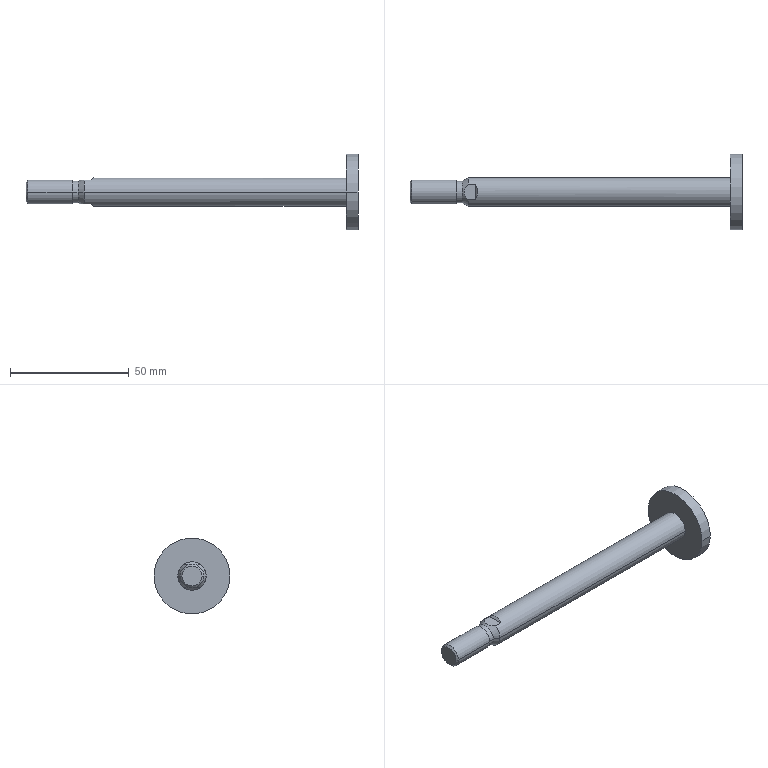Part | SolidWorks | features BaseBody 1 | 1 solid | 20 faces | box 140 x 32 x 32 mm | volume 18387 mm3 | cylinder 8 | plane 8 | cone 4 | commonest cylinder face diameters 9.1 x2 10 x2 12 x2 32 x2
STEP:
#1=CARTESIAN_POINT('',(-40.,4.233,0.));
#2=VERTEX_POINT('',#1);
#3=CARTESIAN_POINT('',(-40.,-4.233,0.));
#4=VERTEX_POINT('',#3);
#5=CARTESIAN_POINT('',(-40.,0.,0.));
#6=DIRECTION('',(1.,0.,0.));
#7=DIRECTION('',(0.,1.,0.));
#8=AXIS2_PLACEMENT_3D('',#5,#6,#7);
#9=CIRCLE('',#8,4.233);
#10=EDGE_CURVE('',#2,#4,#9,.T.);
#11=ORIENTED_EDGE('',*,*,#10,.T.);
#12=CARTESIAN_POINT('',(-39.233,-5.,0.));
#13=VERTEX_POINT('',#12);
#14=CARTESIAN_POINT('',(-40.,-4.233,0.));
#15=DIRECTION('',(0.7071,-0.7071,0.));
#16=VECTOR('',#15,1000.);
#17=LINE('',#14,#16);
#18=EDGE_CURVE('',#4,#13,#17,.T.);
#19=ORIENTED_EDGE('',*,*,#18,.T.);
#20=CARTESIAN_POINT('',(-39.233,5.,0.));
#21=VERTEX_POINT('',#20);
#22=CARTESIAN_POINT('',(-39.233,0.,0.));
#23=DIRECTION('',(1.,0.,0.));
#24=DIRECTION('',(0.,1.,0.));
#25=AXIS2_PLACEMENT_3D('',#22,#23,#24);
#26=CIRCLE('',#25,5.);
#27=EDGE_CURVE('',#21,#13,#26,.T.);
#28=ORIENTED_EDGE('',*,*,#27,.F.);
#29=CARTESIAN_POINT('',(-40.,4.233,0.));
#30=DIRECTION('',(0.7071,0.7071,0.));
#31=VECTOR('',#30,1000.);
#32=LINE('',#29,#31);
#33=EDGE_CURVE('',#2,#21,#32,.T.);
#34=ORIENTED_EDGE('',*,*,#33,.F.);
#35=EDGE_LOOP('',(#11,#19,#28,#34));
#36=FACE_OUTER_BOUND('',#35,.T.);
#37=CARTESIAN_POINT('',(-40.,0.,0.));
#38=DIRECTION('',(1.,0.,0.));
#39=DIRECTION('',(0.,1.,0.));
#40=AXIS2_PLACEMENT_3D('',#37,#38,#39);
#41=CONICAL_SURFACE('',#40,4.233,0.7854);
#42=ADVANCED_FACE('',(#36),#41,.T.);
#43=ORIENTED_EDGE('',*,*,#27,.T.);
#44=CARTESIAN_POINT('',(-20.5,-5.,0.));
#45=VERTEX_POINT('',#44);
#46=CARTESIAN_POINT('',(100.,-5.,0.));
#47=DIRECTION('',(1.,0.,0.));
#48=VECTOR('',#47,1000.);
#49=LINE('',#46,#48);
#50=EDGE_CURVE('',#13,#45,#49,.T.);
#51=ORIENTED_EDGE('',*,*,#50,.T.);
#52=CARTESIAN_POINT('',(-20.5,5.,0.));
#53=VERTEX_POINT('',#52);
#54=CARTESIAN_POINT('',(-20.5,0.,0.));
#55=DIRECTION('',(1.,0.,0.));
#56=DIRECTION('',(0.,1.,0.));
#57=AXIS2_PLACEMENT_3D('',#54,#55,#56);
#58=CIRCLE('',#57,5.);
#59=EDGE_CURVE('',#53,#45,#58,.T.);
#60=ORIENTED_EDGE('',*,*,#59,.F.);
#61=CARTESIAN_POINT('',(100.,5.,0.));
#62=DIRECTION('',(1.,0.,0.));
#63=VECTOR('',#62,1000.);
#64=LINE('',#61,#63);
#65=EDGE_CURVE('',#21,#53,#64,.T.);
#66=ORIENTED_EDGE('',*,*,#65,.F.);
#67=EDGE_LOOP('',(#43,#51,#60,#66));
#68=FACE_OUTER_BOUND('',#67,.T.);
#69=CARTESIAN_POINT('',(100.,0.,0.));
#70=DIRECTION('',(1.,0.,0.));
#71=DIRECTION('',(0.,1.,0.));
#72=AXIS2_PLACEMENT_3D('',#69,#70,#71);
#73=CYLINDRICAL_SURFACE('',#72,5.);
#74=ADVANCED_FACE('',(#68),#73,.T.);
#75=CARTESIAN_POINT('',(95.,16.,0.));
#76=VERTEX_POINT('',#75);
#77=CARTESIAN_POINT('',(95.,-16.,0.));
#78=VERTEX_POINT('',#77);
#79=CARTESIAN_POINT('',(95.,0.,0.));
#80=DIRECTION('',(1.,0.,0.));
#81=DIRECTION('',(0.,1.,0.));
#82=AXIS2_PLACEMENT_3D('',#79,#80,#81);
#83=CIRCLE('',#82,16.);
#84=EDGE_CURVE('',#76,#78,#83,.T.);
#85=ORIENTED_EDGE('',*,*,#84,.T.);
#86=CARTESIAN_POINT('',(100.,-16.,0.));
#87=VERTEX_POINT('',#86);
#88=CARTESIAN_POINT('',(100.,-16.,0.));
#89=DIRECTION('',(1.,0.,0.));
#90=VECTOR('',#89,1000.);
#91=LINE('',#88,#90);
#92=EDGE_CURVE('',#78,#87,#91,.T.);
#93=ORIENTED_EDGE('',*,*,#92,.T.);
#94=CARTESIAN_POINT('',(100.,16.,0.));
#95=VERTEX_POINT('',#94);
#96=CARTESIAN_POINT('',(100.,0.,0.));
#97=DIRECTION('',(1.,0.,0.));
#98=DIRECTION('',(0.,1.,0.));
#99=AXIS2_PLACEMENT_3D('',#96,#97,#98);
#100=CIRCLE('',#99,16.);
#101=EDGE_CURVE('',#95,#87,#100,.T.);
#102=ORIENTED_EDGE('',*,*,#101,.F.);
#103=CARTESIAN_POINT('',(100.,16.,0.));
#104=DIRECTION('',(1.,0.,0.));
#105=VECTOR('',#104,1000.);
#106=LINE('',#103,#105);
#107=EDGE_CURVE('',#76,#95,#106,.T.);
#108=ORIENTED_EDGE('',*,*,#107,.F.);
#109=EDGE_LOOP('',(#85,#93,#102,#108));
#110=FACE_OUTER_BOUND('',#109,.T.);
#111=CARTESIAN_POINT('',(100.,0.,0.));
#112=DIRECTION('',(1.,0.,0.));
#113=DIRECTION('',(0.,1.,0.));
#114=AXIS2_PLACEMENT_3D('',#111,#112,#113);
#115=CYLINDRICAL_SURFACE('',#114,16.);
#116=ADVANCED_FACE('',(#110),#115,.T.);
#117=CARTESIAN_POINT('',(-20.5,4.55,0.));
#118=VERTEX_POINT('',#117);
#119=CARTESIAN_POINT('',(-20.5,-4.55,0.));
#120=VERTEX_POINT('',#119);
#121=CARTESIAN_POINT('',(-20.5,0.,0.));
#122=DIRECTION('',(1.,0.,0.));
#123=DIRECTION('',(0.,1.,0.));
#124=AXIS2_PLACEMENT_3D('',#121,#122,#123);
#125=CIRCLE('',#124,4.55);
#126=EDGE_CURVE('',#118,#120,#125,.T.);
#127=ORIENTED_EDGE('',*,*,#126,.T.);
#128=CARTESIAN_POINT('',(-18.,-4.55,0.));
#129=VERTEX_POINT('',#128);
#130=CARTESIAN_POINT('',(100.,-4.55,0.));
#131=DIRECTION('',(1.,0.,0.));
#132=VECTOR('',#131,1000.);
#133=LINE('',#130,#132);
#134=EDGE_CURVE('',#120,#129,#133,.T.);
#135=ORIENTED_EDGE('',*,*,#134,.T.);
#136=CARTESIAN_POINT('',(-18.,4.55,0.));
#137=VERTEX_POINT('',#136);
#138=CARTESIAN_POINT('',(-18.,0.,0.));
#139=DIRECTION('',(1.,0.,0.));
#140=DIRECTION('',(0.,1.,0.));
#141=AXIS2_PLACEMENT_3D('',#138,#139,#140);
#142=CIRCLE('',#141,4.55);
#143=EDGE_CURVE('',#137,#129,#142,.T.);
#144=ORIENTED_EDGE('',*,*,#143,.F.);
#145=CARTESIAN_POINT('',(100.,4.55,0.));
#146=DIRECTION('',(1.,0.,0.));
#147=VECTOR('',#146,1000.);
#148=LINE('',#145,#147);
#149=EDGE_CURVE('',#118,#137,#148,.T.);
#150=ORIENTED_EDGE('',*,*,#149,.F.);
#151=EDGE_LOOP('',(#127,#135,#144,#150));
#152=FACE_OUTER_BOUND('',#151,.T.);
#153=CARTESIAN_POINT('',(100.,0.,0.));
#154=DIRECTION('',(1.,0.,0.));
#155=DIRECTION('',(0.,1.,0.));
#156=AXIS2_PLACEMENT_3D('',#153,#154,#155);
#157=CYLINDRICAL_SURFACE('',#156,4.55);
#158=ADVANCED_FACE('',(#152),#157,.T.);
#159=CARTESIAN_POINT('',(-15.489,-3.317,5.));
#160=VERTEX_POINT('',#159);
#161=CARTESIAN_POINT('',(-15.489,-6.,0.));
#162=VERTEX_POINT('',#161);
#163=CARTESIAN_POINT('',(-15.489,0.,0.));
#164=DIRECTION('',(1.,0.,0.));
#165=DIRECTION('',(0.,-0.5528,0.8333));
#166=AXIS2_PLACEMENT_3D('',#163,#164,#165);
#167=CIRCLE('',#166,6.);
#168=EDGE_CURVE('',#160,#162,#167,.T.);
#169=ORIENTED_EDGE('',*,*,#168,.T.);
#170=CARTESIAN_POINT('',(95.,-6.,0.));
#171=VERTEX_POINT('',#170);
#172=CARTESIAN_POINT('',(100.,-6.,0.));
#173=DIRECTION('',(1.,0.,0.));
#174=VECTOR('',#173,1000.);
#175=LINE('',#172,#174);
#176=EDGE_CURVE('',#162,#171,#175,.T.);
#177=ORIENTED_EDGE('',*,*,#176,.T.);
#178=CARTESIAN_POINT('',(95.,6.,0.));
#179=VERTEX_POINT('',#178);
#180=CARTESIAN_POINT('',(95.,0.,0.));
#181=DIRECTION('',(1.,0.,0.));
#182=DIRECTION('',(0.,1.,0.));
#183=AXIS2_PLACEMENT_3D('',#180,#181,#182);
#184=CIRCLE('',#183,6.);
#185=EDGE_CURVE('',#179,#171,#184,.T.);
#186=ORIENTED_EDGE('',*,*,#185,.F.);
#187=CARTESIAN_POINT('',(-15.489,6.,0.));
#188=VERTEX_POINT('',#187);
#189=CARTESIAN_POINT('',(100.,6.,0.));
#190=DIRECTION('',(1.,0.,0.));
#191=VECTOR('',#190,1000.);
#192=LINE('',#189,#191);
#193=EDGE_CURVE('',#188,#179,#192,.T.);
#194=ORIENTED_EDGE('',*,*,#193,.F.);
#195=CARTESIAN_POINT('',(-15.489,3.317,5.));
#196=VERTEX_POINT('',#195);
#197=CARTESIAN_POINT('',(-15.489,0.,0.));
#198=DIRECTION('',(1.,0.,0.));
#199=DIRECTION('',(0.,0.5528,-0.8333));
#200=AXIS2_PLACEMENT_3D('',#197,#198,#199);
#201=CIRCLE('',#200,6.);
#202=EDGE_CURVE('',#188,#196,#201,.T.);
#203=ORIENTED_EDGE('',*,*,#202,.T.);
#204=CARTESIAN_POINT('',(-12.5,3.317,5.));
#205=VERTEX_POINT('',#204);
#206=CARTESIAN_POINT('',(-12.5,3.317,5.));
#207=DIRECTION('',(-1.,0.,0.));
#208=VECTOR('',#207,1000.);
#209=LINE('',#206,#208);
#210=EDGE_CURVE('',#205,#196,#209,.T.);
#211=ORIENTED_EDGE('',*,*,#210,.F.);
#212=CARTESIAN_POINT('',(-12.5,-3.317,5.));
#213=VERTEX_POINT('',#212);
#214=CARTESIAN_POINT('',(-12.5,-3.317,5.));
#215=CARTESIAN_POINT('',(-12.338,-3.073,5.162));
#216=CARTESIAN_POINT('',(-12.194,-2.816,5.306));
#217=CARTESIAN_POINT('',(-11.945,-2.287,5.555));
#218=CARTESIAN_POINT('',(-11.84,-2.014,5.66));
#219=CARTESIAN_POINT('',(-11.585,-1.168,5.915));
#220=CARTESIAN_POINT('',(-11.5,-0.6025,6.));
#221=CARTESIAN_POINT('',(-11.5,0.6025,6.));
#222=CARTESIAN_POINT('',(-11.585,1.168,5.915));
#223=CARTESIAN_POINT('',(-11.84,2.014,5.66));
#224=CARTESIAN_POINT('',(-11.945,2.287,5.555));
#225=CARTESIAN_POINT('',(-12.194,2.816,5.306));
#226=CARTESIAN_POINT('',(-12.338,3.073,5.162));
#227=CARTESIAN_POINT('',(-12.5,3.317,5.));
#228=B_SPLINE_CURVE_WITH_KNOTS('',3,(#214,#215,#216,#217,#218,#219,#220,#221,#222,#223,#224,#225,#226,#227),.UNSPECIFIED.,.F.,.F.,(4,2,2,2,2,2,4),(5.697,5.844,5.99,6.283,6.576,6.722,6.869),.UNSPECIFIED.);
#229=EDGE_CURVE('',#213,#205,#228,.T.);
#230=ORIENTED_EDGE('',*,*,#229,.F.);
#231=CARTESIAN_POINT('',(-15.489,-3.317,5.));
#232=DIRECTION('',(1.,0.,0.));
#233=VECTOR('',#232,1000.);
#234=LINE('',#231,#233);
#235=EDGE_CURVE('',#160,#213,#234,.T.);
#236=ORIENTED_EDGE('',*,*,#235,.F.);
#237=EDGE_LOOP('',(#169,#177,#186,#194,#203,#211,#230,#236));
#238=FACE_OUTER_BOUND('',#237,.T.);
#239=CARTESIAN_POINT('',(100.,0.,0.));
#240=DIRECTION('',(1.,0.,0.));
#241=DIRECTION('',(0.,1.,0.));
#242=AXIS2_PLACEMENT_3D('',#239,#240,#241);
#243=CYLINDRICAL_SURFACE('',#242,6.);
#244=ADVANCED_FACE('',(#238),#243,.T.);
#245=ORIENTED_EDGE('',*,*,#143,.T.);
#246=CARTESIAN_POINT('',(-18.,-4.55,0.));
#247=DIRECTION('',(0.866,-0.5,0.));
#248=VECTOR('',#247,1000.);
#249=LINE('',#246,#248);
#250=EDGE_CURVE('',#129,#162,#249,.T.);
#251=ORIENTED_EDGE('',*,*,#250,.T.);
#252=ORIENTED_EDGE('',*,*,#168,.F.);
#253=CARTESIAN_POINT('',(-15.489,3.317,5.));
#254=CARTESIAN_POINT('',(-15.71,3.085,5.));
#255=CARTESIAN_POINT('',(-15.923,2.847,5.));
#256=CARTESIAN_POINT('',(-16.322,2.347,5.));
#257=CARTESIAN_POINT('',(-16.507,2.087,5.));
#258=CARTESIAN_POINT('',(-16.831,1.539,5.));
#259=CARTESIAN_POINT('',(-16.969,1.251,5.));
#260=CARTESIAN_POINT('',(-17.165,0.6406,5.));
#261=CARTESIAN_POINT('',(-17.22,0.3239,5.));
#262=CARTESIAN_POINT('',(-17.221,-0.159,5.));
#263=CARTESIAN_POINT('',(-17.207,-0.3208,5.));
#264=CARTESIAN_POINT('',(-17.155,-0.6364,5.));
#265=CARTESIAN_POINT('',(-17.117,-0.7916,5.));
#266=CARTESIAN_POINT('',(-17.019,-1.097,5.));
#267=CARTESIAN_POINT('',(-16.959,-1.247,5.));
#268=CARTESIAN_POINT('',(-16.824,-1.536,5.));
#269=CARTESIAN_POINT('',(-16.749,-1.677,5.));
#270=CARTESIAN_POINT('',(-16.505,-2.09,5.));
#271=CARTESIAN_POINT('',(-16.319,-2.351,5.));
#272=CARTESIAN_POINT('',(-15.921,-2.849,5.));
#273=CARTESIAN_POINT('',(-15.709,-3.086,5.));
#274=CARTESIAN_POINT('',(-15.489,-3.317,5.));
#275=B_SPLINE_CURVE_WITH_KNOTS('',3,(#253,#254,#255,#256,#257,#258,#259,#260,#261,#262,#263,#264,#265,#266,#267,#268,#269,#270,#271,#272,#273,#274),.UNSPECIFIED.,.F.,.F.,(4,2,2,2,2,2,2,2,2,2,4),(15.099,16.056,17.013,17.97,18.927,19.405,19.884,20.363,20.841,21.798,22.755),.UNSPECIFIED.);
#276=EDGE_CURVE('',#196,#160,#275,.T.);
#277=ORIENTED_EDGE('',*,*,#276,.F.);
#278=ORIENTED_EDGE('',*,*,#202,.F.);
#279=CARTESIAN_POINT('',(-18.,4.55,0.));
#280=DIRECTION('',(0.866,0.5,0.));
#281=VECTOR('',#280,1000.);
#282=LINE('',#279,#281);
#283=EDGE_CURVE('',#137,#188,#282,.T.);
#284=ORIENTED_EDGE('',*,*,#283,.F.);
#285=EDGE_LOOP('',(#245,#251,#252,#277,#278,#284));
#286=FACE_OUTER_BOUND('',#285,.T.);
#287=CARTESIAN_POINT('',(-18.,0.,0.));
#288=DIRECTION('',(1.,0.,0.));
#289=DIRECTION('',(0.,1.,0.));
#290=AXIS2_PLACEMENT_3D('',#287,#288,#289);
#291=CONICAL_SURFACE('',#290,4.55,0.5236);
#292=ADVANCED_FACE('',(#286),#291,.T.);
#293=ORIENTED_EDGE('',*,*,#250,.F.);
#294=CARTESIAN_POINT('',(-18.,0.,0.));
#295=DIRECTION('',(1.,0.,0.));
#296=DIRECTION('',(0.,1.,0.));
#297=AXIS2_PLACEMENT_3D('',#294,#295,#296);
#298=CIRCLE('',#297,4.55);
#299=EDGE_CURVE('',#129,#137,#298,.T.);
#300=ORIENTED_EDGE('',*,*,#299,.T.);
#301=ORIENTED_EDGE('',*,*,#283,.T.);
#302=CARTESIAN_POINT('',(-15.489,3.317,-5.));
#303=VERTEX_POINT('',#302);
#304=CARTESIAN_POINT('',(-15.489,0.,0.));
#305=DIRECTION('',(1.,0.,0.));
#306=DIRECTION('',(0.,0.5528,-0.8333));
#307=AXIS2_PLACEMENT_3D('',#304,#305,#306);
#308=CIRCLE('',#307,6.);
#309=EDGE_CURVE('',#303,#188,#308,.T.);
#310=ORIENTED_EDGE('',*,*,#309,.F.);
#311=CARTESIAN_POINT('',(-15.489,-3.317,-5.));
#312=VERTEX_POINT('',#311);
#313=CARTESIAN_POINT('',(-15.489,-3.317,-5.));
#314=CARTESIAN_POINT('',(-15.71,-3.085,-5.));
#315=CARTESIAN_POINT('',(-15.923,-2.847,-5.));
#316=CARTESIAN_POINT('',(-16.322,-2.347,-5.));
#317=CARTESIAN_POINT('',(-16.507,-2.087,-5.));
#318=CARTESIAN_POINT('',(-16.831,-1.539,-5.));
#319=CARTESIAN_POINT('',(-16.969,-1.251,-5.));
#320=CARTESIAN_POINT('',(-17.165,-0.6406,-5.));
#321=CARTESIAN_POINT('',(-17.22,-0.3239,-5.));
#322=CARTESIAN_POINT('',(-17.221,0.159,-5.));
#323=CARTESIAN_POINT('',(-17.207,0.3208,-5.));
#324=CARTESIAN_POINT('',(-17.155,0.6364,-5.));
#325=CARTESIAN_POINT('',(-17.117,0.7916,-5.));
#326=CARTESIAN_POINT('',(-17.019,1.097,-5.));
#327=CARTESIAN_POINT('',(-16.959,1.247,-5.));
#328=CARTESIAN_POINT('',(-16.824,1.536,-5.));
#329=CARTESIAN_POINT('',(-16.749,1.677,-5.));
#330=CARTESIAN_POINT('',(-16.505,2.09,-5.));
#331=CARTESIAN_POINT('',(-16.319,2.351,-5.));
#332=CARTESIAN_POINT('',(-15.921,2.849,-5.));
#333=CARTESIAN_POINT('',(-15.709,3.086,-5.));
#334=CARTESIAN_POINT('',(-15.489,3.317,-5.));
#335=B_SPLINE_CURVE_WITH_KNOTS('',3,(#313,#314,#315,#316,#317,#318,#319,#320,#321,#322,#323,#324,#325,#326,#327,#328,#329,#330,#331,#332,#333,#334),.UNSPECIFIED.,.F.,.F.,(4,2,2,2,2,2,2,2,2,2,4),(15.099,16.056,17.013,17.97,18.927,19.405,19.884,20.363,20.841,21.798,22.755),.UNSPECIFIED.);
#336=EDGE_CURVE('',#312,#303,#335,.T.);
#337=ORIENTED_EDGE('',*,*,#336,.F.);
#338=CARTESIAN_POINT('',(-15.489,0.,0.));
#339=DIRECTION('',(1.,0.,0.));
#340=DIRECTION('',(0.,-0.5528,0.8333));
#341=AXIS2_PLACEMENT_3D('',#338,#339,#340);
#342=CIRCLE('',#341,6.);
#343=EDGE_CURVE('',#162,#312,#342,.T.);
#344=ORIENTED_EDGE('',*,*,#343,.F.);
#345=EDGE_LOOP('',(#293,#300,#301,#310,#337,#344));
#346=FACE_OUTER_BOUND('',#345,.T.);
#347=CARTESIAN_POINT('',(-18.,0.,0.));
#348=DIRECTION('',(1.,0.,0.));
#349=DIRECTION('',(0.,1.,0.));
#350=AXIS2_PLACEMENT_3D('',#347,#348,#349);
#351=CONICAL_SURFACE('',#350,4.55,0.5236);
#352=ADVANCED_FACE('',(#346),#351,.T.);
#353=ORIENTED_EDGE('',*,*,#176,.F.);
#354=ORIENTED_EDGE('',*,*,#343,.T.);
#355=CARTESIAN_POINT('',(-12.5,-3.317,-5.));
#356=VERTEX_POINT('',#355);
#357=CARTESIAN_POINT('',(-12.5,-3.317,-5.));
#358=DIRECTION('',(-1.,0.,0.));
#359=VECTOR('',#358,1000.);
#360=LINE('',#357,#359);
#361=EDGE_CURVE('',#356,#312,#360,.T.);
#362=ORIENTED_EDGE('',*,*,#361,.F.);
#363=CARTESIAN_POINT('',(-12.5,3.317,-5.));
#364=VERTEX_POINT('',#363);
#365=CARTESIAN_POINT('',(-12.5,3.317,-5.));
#366=CARTESIAN_POINT('',(-12.338,3.073,-5.162));
#367=CARTESIAN_POINT('',(-12.194,2.816,-5.306));
#368=CARTESIAN_POINT('',(-11.945,2.287,-5.555));
#369=CARTESIAN_POINT('',(-11.84,2.014,-5.66));
#370=CARTESIAN_POINT('',(-11.585,1.168,-5.915));
#371=CARTESIAN_POINT('',(-11.5,0.6025,-6.));
#372=CARTESIAN_POINT('',(-11.5,-0.6025,-6.));
#373=CARTESIAN_POINT('',(-11.585,-1.168,-5.915));
#374=CARTESIAN_POINT('',(-11.84,-2.014,-5.66));
#375=CARTESIAN_POINT('',(-11.945,-2.287,-5.555));
#376=CARTESIAN_POINT('',(-12.194,-2.816,-5.306));
#377=CARTESIAN_POINT('',(-12.338,-3.073,-5.162));
#378=CARTESIAN_POINT('',(-12.5,-3.317,-5.));
#379=B_SPLINE_CURVE_WITH_KNOTS('',3,(#365,#366,#367,#368,#369,#370,#371,#372,#373,#374,#375,#376,#377,#378),.UNSPECIFIED.,.F.,.F.,(4,2,2,2,2,2,4),(5.697,5.844,5.99,6.283,6.576,6.722,6.869),.UNSPECIFIED.);
#380=EDGE_CURVE('',#364,#356,#379,.T.);
#381=ORIENTED_EDGE('',*,*,#380,.F.);
#382=CARTESIAN_POINT('',(-15.489,3.317,-5.));
#383=DIRECTION('',(1.,0.,0.));
#384=VECTOR('',#383,1000.);
#385=LINE('',#382,#384);
#386=EDGE_CURVE('',#303,#364,#385,.T.);
#387=ORIENTED_EDGE('',*,*,#386,.F.);
#388=ORIENTED_EDGE('',*,*,#309,.T.);
#389=ORIENTED_EDGE('',*,*,#193,.T.);
#390=CARTESIAN_POINT('',(95.,0.,0.));
#391=DIRECTION('',(1.,0.,0.));
#392=DIRECTION('',(0.,1.,0.));
#393=AXIS2_PLACEMENT_3D('',#390,#391,#392);
#394=CIRCLE('',#393,6.);
#395=EDGE_CURVE('',#171,#179,#394,.T.);
#396=ORIENTED_EDGE('',*,*,#395,.F.);
#397=EDGE_LOOP('',(#353,#354,#362,#381,#387,#388,#389,#396));
#398=FACE_OUTER_BOUND('',#397,.T.);
#399=CARTESIAN_POINT('',(100.,0.,0.));
#400=DIRECTION('',(1.,0.,0.));
#401=DIRECTION('',(0.,1.,0.));
#402=AXIS2_PLACEMENT_3D('',#399,#400,#401);
#403=CYLINDRICAL_SURFACE('',#402,6.);
#404=ADVANCED_FACE('',(#398),#403,.T.);
#405=ORIENTED_EDGE('',*,*,#386,.T.);
#406=CARTESIAN_POINT('',(-12.5,3.317,-5.));
#407=DIRECTION('',(0.,-1.,0.));
#408=VECTOR('',#407,1000.);
#409=LINE('',#406,#408);
#410=EDGE_CURVE('',#364,#356,#409,.T.);
#411=ORIENTED_EDGE('',*,*,#410,.T.);
#412=ORIENTED_EDGE('',*,*,#361,.T.);
#413=ORIENTED_EDGE('',*,*,#336,.T.);
#414=EDGE_LOOP('',(#405,#411,#412,#413));
#415=FACE_OUTER_BOUND('',#414,.T.);
#416=CARTESIAN_POINT('',(-40.,22.,-5.));
#417=DIRECTION('',(0.,0.,-1.));
#418=DIRECTION('',(-1.,0.,0.));
#419=AXIS2_PLACEMENT_3D('',#416,#417,#418);
#420=PLANE('',#419);
#421=ADVANCED_FACE('',(#415),#420,.T.);
#422=ORIENTED_EDGE('',*,*,#235,.T.);
#423=CARTESIAN_POINT('',(-12.5,3.317,5.));
#424=DIRECTION('',(0.,-1.,0.));
#425=VECTOR('',#424,1000.);
#426=LINE('',#423,#425);
#427=EDGE_CURVE('',#205,#213,#426,.T.);
#428=ORIENTED_EDGE('',*,*,#427,.F.);
#429=ORIENTED_EDGE('',*,*,#210,.T.);
#430=ORIENTED_EDGE('',*,*,#276,.T.);
#431=EDGE_LOOP('',(#422,#428,#429,#430));
#432=FACE_OUTER_BOUND('',#431,.T.);
#433=CARTESIAN_POINT('',(-12.5,22.,5.));
#434=DIRECTION('',(0.,0.,1.));
#435=DIRECTION('',(1.,0.,0.));
#436=AXIS2_PLACEMENT_3D('',#433,#434,#435);
#437=PLANE('',#436);
#438=ADVANCED_FACE('',(#432),#437,.T.);
#439=ORIENTED_EDGE('',*,*,#134,.F.);
#440=CARTESIAN_POINT('',(-20.5,0.,0.));
#441=DIRECTION('',(1.,0.,0.));
#442=DIRECTION('',(0.,1.,0.));
#443=AXIS2_PLACEMENT_3D('',#440,#441,#442);
#444=CIRCLE('',#443,4.55);
#445=EDGE_CURVE('',#120,#118,#444,.T.);
#446=ORIENTED_EDGE('',*,*,#445,.T.);
#447=ORIENTED_EDGE('',*,*,#149,.T.);
#448=ORIENTED_EDGE('',*,*,#299,.F.);
#449=EDGE_LOOP('',(#439,#446,#447,#448));
#450=FACE_OUTER_BOUND('',#449,.T.);
#451=CARTESIAN_POINT('',(100.,0.,0.));
#452=DIRECTION('',(1.,0.,0.));
#453=DIRECTION('',(0.,1.,0.));
#454=AXIS2_PLACEMENT_3D('',#451,#452,#453);
#455=CYLINDRICAL_SURFACE('',#454,4.55);
#456=ADVANCED_FACE('',(#450),#455,.T.);
#457=ORIENTED_EDGE('',*,*,#84,.F.);
#458=CARTESIAN_POINT('',(95.,0.,0.));
#459=DIRECTION('',(1.,0.,0.));
#460=DIRECTION('',(0.,1.,0.));
#461=AXIS2_PLACEMENT_3D('',#458,#459,#460);
#462=CIRCLE('',#461,16.);
#463=EDGE_CURVE('',#78,#76,#462,.T.);
#464=ORIENTED_EDGE('',*,*,#463,.F.);
#465=EDGE_LOOP('',(#457,#464));
#466=FACE_OUTER_BOUND('',#465,.T.);
#467=ORIENTED_EDGE('',*,*,#185,.T.);
#468=ORIENTED_EDGE('',*,*,#395,.T.);
#469=EDGE_LOOP('',(#467,#468));
#470=FACE_BOUND('',#469,.T.);
#471=CARTESIAN_POINT('',(95.,6.,0.));
#472=DIRECTION('',(1.,0.,0.));
#473=DIRECTION('',(0.,1.,0.));
#474=AXIS2_PLACEMENT_3D('',#471,#472,#473);
#475=PLANE('',#474);
#476=ADVANCED_FACE('',(#466,#470),#475,.F.);
#477=ORIENTED_EDGE('',*,*,#380,.T.);
#478=ORIENTED_EDGE('',*,*,#410,.F.);
#479=EDGE_LOOP('',(#477,#478));
#480=FACE_OUTER_BOUND('',#479,.T.);
#481=CARTESIAN_POINT('',(-12.5,22.,-5.));
#482=DIRECTION('',(-0.7071,0.,-0.7071));
#483=DIRECTION('',(-0.7071,0.,0.7071));
#484=AXIS2_PLACEMENT_3D('',#481,#482,#483);
#485=PLANE('',#484);
#486=ADVANCED_FACE('',(#480),#485,.T.);
#487=ORIENTED_EDGE('',*,*,#229,.T.);
#488=ORIENTED_EDGE('',*,*,#427,.T.);
#489=EDGE_LOOP('',(#487,#488));
#490=FACE_OUTER_BOUND('',#489,.T.);
#491=CARTESIAN_POINT('',(-7.5,22.,10.));
#492=DIRECTION('',(-0.7071,0.,0.7071));
#493=DIRECTION('',(0.7071,0.,0.7071));
#494=AXIS2_PLACEMENT_3D('',#491,#492,#493);
#495=PLANE('',#494);
#496=ADVANCED_FACE('',(#490),#495,.T.);
#497=ORIENTED_EDGE('',*,*,#126,.F.);
#498=ORIENTED_EDGE('',*,*,#445,.F.);
#499=EDGE_LOOP('',(#497,#498));
#500=FACE_BOUND('',#499,.T.);
#501=ORIENTED_EDGE('',*,*,#59,.T.);
#502=CARTESIAN_POINT('',(-20.5,0.,0.));
#503=DIRECTION('',(1.,0.,0.));
#504=DIRECTION('',(0.,1.,0.));
#505=AXIS2_PLACEMENT_3D('',#502,#503,#504);
#506=CIRCLE('',#505,5.);
#507=EDGE_CURVE('',#45,#53,#506,.T.);
#508=ORIENTED_EDGE('',*,*,#507,.T.);
#509=EDGE_LOOP('',(#501,#508));
#510=FACE_OUTER_BOUND('',#509,.T.);
#511=CARTESIAN_POINT('',(-20.5,5.,0.));
#512=DIRECTION('',(-1.,0.,0.));
#513=DIRECTION('',(0.,-1.,0.));
#514=AXIS2_PLACEMENT_3D('',#511,#512,#513);
#515=PLANE('',#514);
#516=ADVANCED_FACE('',(#500,#510),#515,.F.);
#517=ORIENTED_EDGE('',*,*,#92,.F.);
#518=ORIENTED_EDGE('',*,*,#463,.T.);
#519=ORIENTED_EDGE('',*,*,#107,.T.);
#520=CARTESIAN_POINT('',(100.,0.,0.));
#521=DIRECTION('',(1.,0.,0.));
#522=DIRECTION('',(0.,1.,0.));
#523=AXIS2_PLACEMENT_3D('',#520,#521,#522);
#524=CIRCLE('',#523,16.);
#525=EDGE_CURVE('',#87,#95,#524,.T.);
#526=ORIENTED_EDGE('',*,*,#525,.F.);
#527=EDGE_LOOP('',(#517,#518,#519,#526));
#528=FACE_OUTER_BOUND('',#527,.T.);
#529=CARTESIAN_POINT('',(100.,0.,0.));
#530=DIRECTION('',(1.,0.,0.));
#531=DIRECTION('',(0.,1.,0.));
#532=AXIS2_PLACEMENT_3D('',#529,#530,#531);
#533=CYLINDRICAL_SURFACE('',#532,16.);
#534=ADVANCED_FACE('',(#528),#533,.T.);
#535=ORIENTED_EDGE('',*,*,#50,.F.);
#536=CARTESIAN_POINT('',(-39.233,0.,0.));
#537=DIRECTION('',(1.,0.,0.));
#538=DIRECTION('',(0.,1.,0.));
#539=AXIS2_PLACEMENT_3D('',#536,#537,#538);
#540=CIRCLE('',#539,5.);
#541=EDGE_CURVE('',#13,#21,#540,.T.);
#542=ORIENTED_EDGE('',*,*,#541,.T.);
#543=ORIENTED_EDGE('',*,*,#65,.T.);
#544=ORIENTED_EDGE('',*,*,#507,.F.);
#545=EDGE_LOOP('',(#535,#542,#543,#544));
#546=FACE_OUTER_BOUND('',#545,.T.);
#547=CARTESIAN_POINT('',(100.,0.,0.));
#548=DIRECTION('',(1.,0.,0.));
#549=DIRECTION('',(0.,1.,0.));
#550=AXIS2_PLACEMENT_3D('',#547,#548,#549);
#551=CYLINDRICAL_SURFACE('',#550,5.);
#552=ADVANCED_FACE('',(#546),#551,.T.);
#553=ORIENTED_EDGE('',*,*,#101,.T.);
#554=ORIENTED_EDGE('',*,*,#525,.T.);
#555=EDGE_LOOP('',(#553,#554));
#556=FACE_OUTER_BOUND('',#555,.T.);
#557=CARTESIAN_POINT('',(100.,16.,0.));
#558=DIRECTION('',(-1.,0.,0.));
#559=DIRECTION('',(0.,-1.,0.));
#560=AXIS2_PLACEMENT_3D('',#557,#558,#559);
#561=PLANE('',#560);
#562=ADVANCED_FACE('',(#556),#561,.F.);
#563=ORIENTED_EDGE('',*,*,#18,.F.);
#564=CARTESIAN_POINT('',(-40.,0.,0.));
#565=DIRECTION('',(1.,0.,0.));
#566=DIRECTION('',(0.,1.,0.));
#567=AXIS2_PLACEMENT_3D('',#564,#565,#566);
#568=CIRCLE('',#567,4.233);
#569=EDGE_CURVE('',#4,#2,#568,.T.);
#570=ORIENTED_EDGE('',*,*,#569,.T.);
#571=ORIENTED_EDGE('',*,*,#33,.T.);
#572=ORIENTED_EDGE('',*,*,#541,.F.);
#573=EDGE_LOOP('',(#563,#570,#571,#572));
#574=FACE_OUTER_BOUND('',#573,.T.);
#575=CARTESIAN_POINT('',(-40.,0.,0.));
#576=DIRECTION('',(1.,0.,0.));
#577=DIRECTION('',(0.,1.,0.));
#578=AXIS2_PLACEMENT_3D('',#575,#576,#577);
#579=CONICAL_SURFACE('',#578,4.233,0.7854);
#580=ADVANCED_FACE('',(#574),#579,.T.);
#581=ORIENTED_EDGE('',*,*,#10,.F.);
#582=ORIENTED_EDGE('',*,*,#569,.F.);
#583=EDGE_LOOP('',(#581,#582));
#584=FACE_OUTER_BOUND('',#583,.T.);
#585=CARTESIAN_POINT('',(-40.,0.,0.));
#586=DIRECTION('',(1.,0.,0.));
#587=DIRECTION('',(0.,1.,0.));
#588=AXIS2_PLACEMENT_3D('',#585,#586,#587);
#589=PLANE('',#588);
#590=ADVANCED_FACE('',(#584),#589,.F.);
#591=CLOSED_SHELL('',(#42,#74,#116,#158,#244,#292,#352,#404,#421,#438,#456,#476,#486,#496,#516,#534,#552,#562,#580,#590));
#592=MANIFOLD_SOLID_BREP('',#591);
#593=CARTESIAN_POINT('',(0.,0.,0.));
#594=DIRECTION('',(0.,0.,1.));
#595=DIRECTION('',(1.,0.,0.));
#596=AXIS2_PLACEMENT_3D('',#593,#594,#595);
#597=(LENGTH_UNIT()NAMED_UNIT(*)SI_UNIT(.MILLI.,.METRE.));
#598=UNCERTAINTY_MEASURE_WITH_UNIT(LENGTH_MEASURE(0.00001),#597,'','');
#599=(NAMED_UNIT(*)PLANE_ANGLE_UNIT()SI_UNIT($,.RADIAN.));
#600=(NAMED_UNIT(*)SI_UNIT($,.STERADIAN.)SOLID_ANGLE_UNIT());
#601=(GEOMETRIC_REPRESENTATION_CONTEXT(3)GLOBAL_UNCERTAINTY_ASSIGNED_CONTEXT((#598))GLOBAL_UNIT_ASSIGNED_CONTEXT((#597,#599,#600))REPRESENTATION_CONTEXT('',''));
#602=ADVANCED_BREP_SHAPE_REPRESENTATION('',(#592,#596),#601);